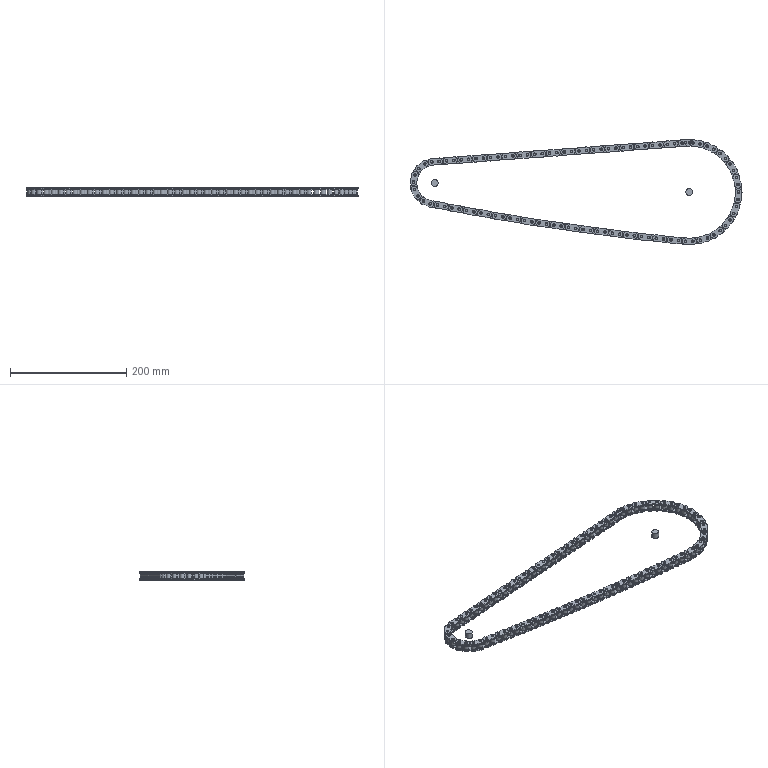Part | SolidWorks | features BaseBody 152 | 152 solids | 3008 faces | volume 137821 mm3 | cylinder 2004 | plane 604 | cone 400 | commonest cylinder face diameters 4.45 x800 11.81 x600 57.066 x400 8.51 x200 12 x4